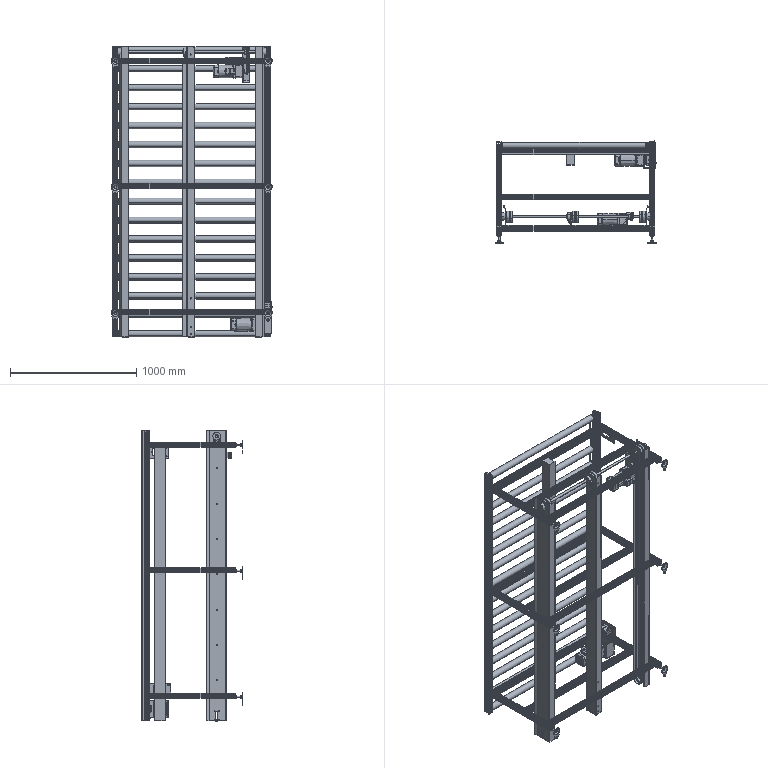Part | SolidWorks | features ReferencePattern 34, LocalLPattern 3 | 108 solids | 12245 faces | volume 74187256 mm3 | plane 5485 | cylinder 3749 | spline 1885 | cone 1007 | torus 78 | sphere 41 | commonest cylinder face diameters 1 x478 43 x354 4.45 x256 9 x240 8 x152 6.8 x150